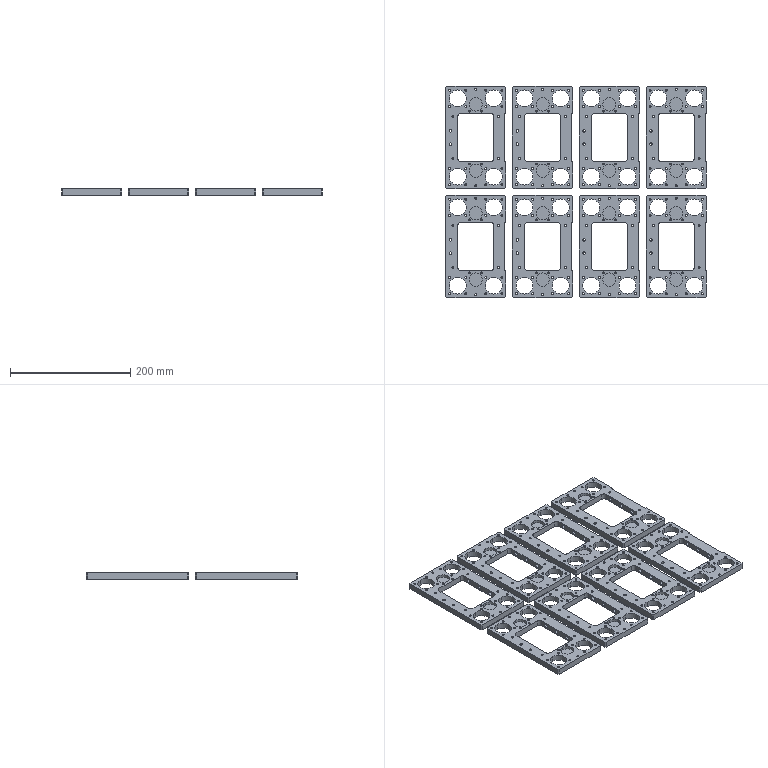NC program | NX | posted with a generic post | part box 433 x 351 x 10 mm
Lines 10233 to 11306 of 15742:
(PLANAR_MILL_COPY_COPY_COPY , TOOL : D6A45)
N20428 T01 M6
N20430 G54
N20432 G17 G0 G90 X26.9 Y-89.634 B0. C0. S9500 M3
N20434 G43 Z30. H1
N20436 Z0.5
N20438 G94 G1 Z-1. F1250.
N20440 G3 X26.4 Y-90.5 R1.
N20442 G1 Y-125.5
N20444 G3 X30.5 Y-129.6 R4.1
N20446 G1 X80.5
N20448 G3 X84.6 Y-125.5 R4.1
N20450 G1 Y-55.5
N20452 G3 X80.5 Y-51.4 R4.1
N20454 G1 X30.5
N20456 G3 X26.4 Y-55.5 R4.1
N20458 G1 Y-90.5
N20460 G3 X26.9 Y-91.366 R1.
N20462 G1 Z0.5
N20464 G0 Z30.
N20466 X4.1
N20468 Z0.5
N20470 G1 Z-1.
N20472 G3 X4.6 Y-90.5 R1.
N20474 G1 Y-7.5
N20476 G2 X4.864 Y-6.864 R0.9
N20478 G1 X6.864 Y-4.864
N20480 G2 X7.5 Y-4.6 R0.9
N20482 G1 X103.5
N20484 G2 X104.136 Y-4.864 R0.9
N20486 G1 X106.136 Y-6.864
N20488 G2 X106.4 Y-7.5 R0.9
N20490 G1 Y-50.5
N20492 G2 X105.5 Y-51.4 R0.9
N20494 G1 X104.4
N20496 Y-129.6
N20498 X105.5
N20500 G2 X106.4 Y-130.5 R0.9
N20502 G1 Y-173.5
N20504 G2 X106.136 Y-174.136 R0.9
N20506 G1 X104.136 Y-176.136
N20508 G2 X103.5 Y-176.4 R0.9
N20510 G1 X7.5
N20512 G2 X6.864 Y-176.136 R0.9
N20514 G1 X4.864 Y-174.136
N20516 G2 X4.6 Y-173.5 R0.9
N20518 G1 Y-90.5
N20520 G3 X4.1 Y-89.634 R1.
N20522 G1 Z0.5
N20524 G0 Z30.
N20526 X12.634 Y-102.2
N20528 Z0.5
N20530 G1 Z-1.
N20532 G3 X13.5 Y-102.7 R1.
N20534 X14.7 Y-101.5 R1.2
N20536 X13.5 Y-102.7 R-1.2
N20538 X14.366 Y-102.2 R1.
N20540 G1 Z0.5
N20542 G0 Z30.
N20544 X12.634 Y-80.2
N20546 Z0.5
N20548 G1 Z-1.
N20550 G3 X13.5 Y-80.7 R1.
N20552 X14.7 Y-79.5 R1.2
N20554 X13.5 Y-80.7 R-1.2
N20556 X14.366 Y-80.2 R1.
N20558 G1 Z0.5
N20560 G0 Z30.
N20562 X17.067 Y-56.
N20564 Z0.5
N20566 G1 Z-1.
N20568 G3 X17.5 Y-56.25 R0.5
N20570 X18.25 Y-55.5 R0.75
N20572 X17.5 Y-56.25 R-0.75
N20574 X17.933 Y-56. R0.5
N20576 G1 Z0.5
N20578 G0 Z30.
N20580 X11.632 Y-39.435
N20582 Z0.5
N20584 G1 Z-1.
N20586 G3 X12.065 Y-39.685 R0.5
N20588 X12.815 Y-38.935 R0.75
N20590 X12.065 Y-39.685 R-0.75
N20592 X12.498 Y-39.435 R0.5
N20594 G1 Z0.5
N20596 G0 Z30.
N20598 X-12.498
N20600 Z0.5
N20602 G1 Z-1.
N20604 G3 X-12.065 Y-39.685 R0.5
N20606 X-11.315 Y-38.935 R0.75
N20608 X-12.065 Y-39.685 R-0.75
N20610 X-11.632 Y-39.435 R0.5
N20612 G1 Z0.5
N20614 G0 Z30.
N20616 X-17.933 Y-56.
N20618 Z0.5
N20620 G1 Z-1.
N20622 G3 X-17.5 Y-56.25 R0.5
N20624 X-16.75 Y-55.5 R0.75
N20626 X-17.5 Y-56.25 R-0.75
N20628 X-17.067 Y-56. R0.5
N20630 G1 Z0.5
N20632 G0 Z30.
N20634 X-39.368 Y-39.435
N20636 Z0.5
N20638 G1 Z-1.
N20640 G3 X-38.935 Y-39.685 R0.5
N20642 X-38.185 Y-38.935 R0.75
N20644 X-38.935 Y-39.685 R-0.75
N20646 X-38.502 Y-39.435 R0.5
N20648 G1 Z0.5
N20650 G0 Z30.
N20652 X-45.933 Y-47.
N20654 Z0.5
N20656 G1 Z-1.
N20658 G3 X-45.5 Y-47.25 R0.5
N20660 X-44.75 Y-46.5 R0.75
N20662 X-45.5 Y-47.25 R-0.75
N20664 X-45.067 Y-47. R0.5
N20666 G1 Z0.5
N20668 G0 Z30.
N20670 X-56.366 Y-45.1
N20672 Z0.5
N20674 G1 Z-1.
N20676 G3 X-55.5 Y-45.6 R1.
N20678 X-45.4 Y-35.5 R10.1
N20680 X-55.5 Y-45.6 R-10.1
N20682 X-54.634 Y-45.1 R1.
N20684 G1 Z0.5
N20686 G0 Z30.
N20688 X-72.498 Y-39.435
N20690 Z0.5
N20692 G1 Z-1.
N20694 G3 X-72.065 Y-39.685 R0.5
N20696 X-71.315 Y-38.935 R0.75
N20698 X-72.065 Y-39.685 R-0.75
N20700 X-71.632 Y-39.435 R0.5
N20702 G1 Z0.5
N20704 G0 Z30.
N20706 X-65.933 Y-47.
N20708 Z0.5
N20710 G1 Z-1.
N20712 G3 X-65.5 Y-47.25 R0.5
N20714 X-64.75 Y-46.5 R0.75
N20716 X-65.5 Y-47.25 R-0.75
N20718 X-65.067 Y-47. R0.5
N20720 G1 Z0.5
N20722 G0 Z30.
N20724 X-84.1 Y-89.634
N20726 Z0.5
N20728 G1 Z-1.
N20730 G3 X-84.6 Y-90.5 R1.
N20732 G1 Y-125.5
N20734 G3 X-80.5 Y-129.6 R4.1
N20736 G1 X-30.5
N20738 G3 X-26.4 Y-125.5 R4.1
N20740 G1 Y-55.5
N20742 G3 X-30.5 Y-51.4 R4.1
N20744 G1 X-80.5
N20746 G3 X-84.6 Y-55.5 R4.1
N20748 G1 Y-90.5
N20750 G3 X-84.1 Y-91.366 R1.
N20752 G1 Z0.5
N20754 G0 Z30.
N20756 X-106.9
N20758 Z0.5
N20760 G1 Z-1.
N20762 G3 X-106.4 Y-90.5 R1.
N20764 G1 Y-7.5
N20766 G2 X-106.136 Y-6.864 R0.9
N20768 G1 X-104.136 Y-4.864
N20770 G2 X-103.5 Y-4.6 R0.9
N20772 G1 X-7.5
N20774 G2 X-6.864 Y-4.864 R0.9
N20776 G1 X-4.864 Y-6.864
N20778 G2 X-4.6 Y-7.5 R0.9
N20780 G1 Y-50.5
N20782 G2 X-5.5 Y-51.4 R0.9
N20784 G1 X-6.6
N20786 Y-129.6
N20788 X-5.5
N20790 G2 X-4.6 Y-130.5 R0.9
N20792 G1 Y-173.5
N20794 G2 X-4.864 Y-174.136 R0.9
N20796 G1 X-6.864 Y-176.136
N20798 G2 X-7.5 Y-176.4 R0.9
N20800 G1 X-103.5
N20802 G2 X-104.136 Y-176.136 R0.9
N20804 G1 X-106.136 Y-174.136
N20806 G2 X-106.4 Y-173.5 R0.9
N20808 G1 Y-90.5
N20810 G3 X-106.9 Y-89.634 R1.
N20812 G1 Z0.5
N20814 G0 Z30.
N20816 X-98.366 Y-80.2
N20818 Z0.5
N20820 G1 Z-1.
N20822 G3 X-97.5 Y-80.7 R1.
N20824 X-96.3 Y-79.5 R1.2
N20826 X-97.5 Y-80.7 R-1.2
N20828 X-96.634 Y-80.2 R1.
N20830 G1 Z0.5
N20832 G0 Z30.
N20834 X-98.366 Y-102.2
N20836 Z0.5
N20838 G1 Z-1.
N20840 G3 X-97.5 Y-102.7 R1.
N20842 X-96.3 Y-101.5 R1.2
N20844 X-97.5 Y-102.7 R-1.2
N20846 X-96.634 Y-102.2 R1.
N20848 G1 Z0.5
N20850 G0 Z30.
N20852 X-93.933 Y-126.
N20854 Z0.5
N20856 G1 Z-1.
N20858 G3 X-93.5 Y-126.25 R0.5
N20860 X-92.75 Y-125.5 R0.75
N20862 X-93.5 Y-126.25 R-0.75
N20864 X-93.067 Y-126. R0.5
N20866 G1 Z0.5
N20868 G0 Z30.
N20870 X-99.368 Y-142.565
N20872 Z0.5
N20874 G1 Z-1.
N20876 G3 X-98.935 Y-142.815 R0.5
N20878 X-98.185 Y-142.065 R0.75
N20880 X-98.935 Y-142.815 R-0.75
N20882 X-98.502 Y-142.565 R0.5
N20884 G1 Z0.5
N20886 G0 Z30.
N20888 X-86.366 Y-168.15
N20890 Z0.5
N20892 G1 Z-1.
N20894 G3 X-85.5 Y-168.65 R1.
N20896 X-72.35 Y-155.5 R13.15
N20898 X-85.5 Y-168.65 R-13.15
N20900 X-84.634 Y-168.15 R1.
N20902 G1 Z0.5
N20904 G0 Z30.
N20906 X-72.498 Y-142.565
N20908 Z0.5
N20910 G1 Z-1.
N20912 G3 X-72.065 Y-142.815 R0.5
N20914 X-71.315 Y-142.065 R0.75
N20916 X-72.065 Y-142.815 R-0.75
N20918 X-71.632 Y-142.565 R0.5
N20920 G1 Z0.5
N20922 G0 Z30.
N20924 X-65.933 Y-135.
N20926 Z0.5
N20928 G1 Z-1.
N20930 G3 X-65.5 Y-135.25 R0.5
N20932 X-64.75 Y-134.5 R0.75
N20934 X-65.5 Y-135.25 R-0.75
N20936 X-65.067 Y-135. R0.5
N20938 G1 Z0.5
N20940 G0 Z30.
N20942 X-56.366 Y-155.1
N20944 Z0.5
N20946 G1 Z-1.
N20948 G3 X-55.5 Y-155.6 R1.
N20950 X-45.4 Y-145.5 R10.1
N20952 X-55.5 Y-155.6 R-10.1
N20954 X-54.634 Y-155.1 R1.
N20956 G1 Z0.5
N20958 G0 Z30.
N20960 X-45.933 Y-135.
N20962 Z0.5
N20964 G1 Z-1.
N20966 G3 X-45.5 Y-135.25 R0.5
N20968 X-44.75 Y-134.5 R0.75
N20970 X-45.5 Y-135.25 R-0.75
N20972 X-45.067 Y-135. R0.5
N20974 G1 Z0.5
N20976 G0 Z30.
N20978 X-39.368 Y-142.565
N20980 Z0.5
N20982 G1 Z-1.
N20984 G3 X-38.935 Y-142.815 R0.5
N20986 X-38.185 Y-142.065 R0.75
N20988 X-38.935 Y-142.815 R-0.75
N20990 X-38.502 Y-142.565 R0.5
N20992 G1 Z0.5
N20994 G0 Z30.
N20996 X-17.933 Y-126.
N20998 Z0.5
N21000 G1 Z-1.
N21002 G3 X-17.5 Y-126.25 R0.5
N21004 X-16.75 Y-125.5 R0.75
N21006 X-17.5 Y-126.25 R-0.75
N21008 X-17.067 Y-126. R0.5
N21010 G1 Z0.5
N21012 G0 Z30.
N21014 X-12.498 Y-142.565
N21016 Z0.5
N21018 G1 Z-1.
N21020 G3 X-12.065 Y-142.815 R0.5
N21022 X-11.315 Y-142.065 R0.75
N21024 X-12.065 Y-142.815 R-0.75
N21026 X-11.632 Y-142.565 R0.5
N21028 G1 Z0.5
N21030 G0 Z30.
N21032 X17.067 Y-126.
N21034 Z0.5
N21036 G1 Z-1.
N21038 G3 X17.5 Y-126.25 R0.5
N21040 X18.25 Y-125.5 R0.75
N21042 X17.5 Y-126.25 R-0.75
N21044 X17.933 Y-126. R0.5
N21046 G1 Z0.5
N21048 G0 Z30.
N21050 X11.632 Y-142.565
N21052 Z0.5
N21054 G1 Z-1.
N21056 G3 X12.065 Y-142.815 R0.5
N21058 X12.815 Y-142.065 R0.75
N21060 X12.065 Y-142.815 R-0.75
N21062 X12.498 Y-142.565 R0.5
N21064 G1 Z0.5
N21066 G0 Z30.
N21068 X24.634 Y-168.15
N21070 Z0.5
N21072 G1 Z-1.
N21074 G3 X25.5 Y-168.65 R1.
N21076 X38.65 Y-155.5 R13.15
N21078 X25.5 Y-168.65 R-13.15
N21080 X26.366 Y-168.15 R1.
N21082 G1 Z0.5
N21084 G0 Z30.
N21086 X38.502 Y-142.565
N21088 Z0.5
N21090 G1 Z-1.
N21092 G3 X38.935 Y-142.815 R0.5
N21094 X39.685 Y-142.065 R0.75
N21096 X38.935 Y-142.815 R-0.75
N21098 X39.368 Y-142.565 R0.5
N21100 G1 Z0.5
N21102 G0 Z30.
N21104 X45.067 Y-135.
N21106 Z0.5
N21108 G1 Z-1.
N21110 G3 X45.5 Y-135.25 R0.5
N21112 X46.25 Y-134.5 R0.75
N21114 X45.5 Y-135.25 R-0.75
N21116 X45.933 Y-135. R0.5
N21118 G1 Z0.5
N21120 G0 Z30.
N21122 X54.634 Y-155.1
N21124 Z0.5
N21126 G1 Z-1.
N21128 G3 X55.5 Y-155.6 R1.
N21130 X65.6 Y-145.5 R10.1
N21132 X55.5 Y-155.6 R-10.1
N21134 X56.366 Y-155.1 R1.
N21136 G1 Z0.5
N21138 G0 Z30.
N21140 X65.067 Y-135.
N21142 Z0.5
N21144 G1 Z-1.
N21146 G3 X65.5 Y-135.25 R0.5
N21148 X66.25 Y-134.5 R0.75
N21150 X65.5 Y-135.25 R-0.75
N21152 X65.933 Y-135. R0.5
N21154 G1 Z0.5
N21156 G0 Z30.
N21158 X71.632 Y-142.565
N21160 Z0.5
N21162 G1 Z-1.
N21164 G3 X72.065 Y-142.815 R0.5
N21166 X72.815 Y-142.065 R0.75
N21168 X72.065 Y-142.815 R-0.75
N21170 X72.498 Y-142.565 R0.5
N21172 G1 Z0.5
N21174 G0 Z30.
N21176 X98.502
N21178 Z0.5
N21180 G1 Z-1.
N21182 G3 X98.935 Y-142.815 R0.5
N21184 X99.685 Y-142.065 R0.75
N21186 X98.935 Y-142.815 R-0.75
N21188 X99.368 Y-142.565 R0.5
N21190 G1 Z0.5
N21192 G0 Z30.
N21194 X93.067 Y-126.
N21196 Z0.5
N21198 G1 Z-1.
N21200 G3 X93.5 Y-126.25 R0.5
N21202 X94.25 Y-125.5 R0.75
N21204 X93.5 Y-126.25 R-0.75
N21206 X93.933 Y-126. R0.5
N21208 G1 Z0.5
N21210 G0 Z30.
N21212 X122.632 Y-142.565
N21214 Z0.5
N21216 G1 Z-1.
N21218 G3 X123.065 Y-142.815 R0.5
N21220 X123.815 Y-142.065 R0.75
N21222 X123.065 Y-142.815 R-0.75
N21224 X123.498 Y-142.565 R0.5
N21226 G1 Z0.5
N21228 G0 Z30.
N21230 X128.067 Y-126.
N21232 Z0.5
N21234 G1 Z-1.
N21236 G3 X128.5 Y-126.25 R0.5
N21238 X129.25 Y-125.5 R0.75
N21240 X128.5 Y-126.25 R-0.75
N21242 X128.933 Y-126. R0.5
N21244 G1 Z0.5
N21246 G0 Z30.
N21248 X123.634 Y-102.2
N21250 Z0.5
N21252 G1 Z-1.
N21254 G3 X124.5 Y-102.7 R1.
N21256 X125.7 Y-101.5 R1.2
N21258 X124.5 Y-102.7 R-1.2
N21260 X125.366 Y-102.2 R1.
N21262 G1 Z0.5
N21264 G0 Z30.
N21266 X125.2 Y-80.366
N21268 Z0.5
N21270 G1 Z-1.
N21272 G3 X125.7 Y-79.5 R1.
N21274 X124.5 Y-78.3 R1.2
N21276 X125.7 Y-79.5 R-1.2
N21278 X125.2 Y-78.634 R1.
N21280 G1 Z0.5
N21282 G0 Z30.
N21284 X129. Y-55.933
N21286 Z0.5
N21288 G1 Z-1.
N21290 G3 X129.25 Y-55.5 R0.5
N21292 X128.5 Y-54.75 R0.75
N21294 X129.25 Y-55.5 R-0.75
N21296 X129. Y-55.067 R0.5
N21298 G1 Z0.5
N21300 G0 Z30.
N21302 X123.565 Y-39.368
N21304 Z0.5
N21306 G1 Z-1.
N21308 G3 X123.815 Y-38.935 R0.5
N21310 X123.065 Y-38.185 R0.75
N21312 X123.815 Y-38.935 R-0.75
N21314 X123.565 Y-38.502 R0.5
N21316 G1 Z0.5
N21318 G0 Z30.
N21320 X149.15 Y-26.366
N21322 Z0.5
N21324 G1 Z-1.
N21326 G3 X149.65 Y-25.5 R1.
N21328 X136.5 Y-12.35 R13.15
N21330 X149.65 Y-25.5 R-13.15
N21332 X149.15 Y-24.634 R1.
N21334 G1 Z0.5
N21336 G0 Z30.
N21338 X123.565 Y-12.498
N21340 Z0.5
N21342 G1 Z-1.
N21344 G3 X123.815 Y-12.065 R0.5
N21346 X123.065 Y-11.315 R0.75
N21348 X123.815 Y-12.065 R-0.75
N21350 X123.565 Y-11.632 R0.5
N21352 G1 Z0.5
N21354 G0 Z30.
N21356 Y11.632
N21358 Z0.5
N21360 G1 Z-1.
N21362 G3 X123.815 Y12.065 R0.5
N21364 X123.065 Y12.815 R0.75
N21366 X123.815 Y12.065 R-0.75
N21368 X123.565 Y12.498 R0.5
N21370 G1 Z0.5
N21372 G0 Z30.
N21374 X99.435 Y11.632
N21376 Z0.5
N21378 G1 Z-1.
N21380 G3 X99.685 Y12.065 R0.5
N21382 X98.935 Y12.815 R0.75
N21384 X99.685 Y12.065 R-0.75
N21386 X99.435 Y12.498 R0.5
N21388 G1 Z0.5
N21390 G0 Z30.
N21392 Y-12.498
N21394 Z0.5
N21396 G1 Z-1.
N21398 G3 X99.685 Y-12.065 R0.5
N21400 X98.935 Y-11.315 R0.75
N21402 X99.685 Y-12.065 R-0.75
N21404 X99.435 Y-11.632 R0.5
N21406 G1 Z0.5
N21408 G0 Z30.
N21410 X98.15 Y-26.366
N21412 Z0.5
N21414 G1 Z-1.
N21416 G3 X98.65 Y-25.5 R1.
N21418 X85.5 Y-12.35 R13.15
N21420 X98.65 Y-25.5 R-13.15
N21422 X98.15 Y-24.634 R1.
N21424 G1 Z0.5
N21426 G0 Z30.
N21428 X99.435 Y-39.368
N21430 Z0.5
N21432 G1 Z-1.
N21434 G3 X99.685 Y-38.935 R0.5
N21436 X98.935 Y-38.185 R0.75
N21438 X99.685 Y-38.935 R-0.75
N21440 X99.435 Y-38.502 R0.5
N21442 G1 Z0.5
N21444 G0 Z30.
N21446 X93.067 Y-56.
N21448 Z0.5
N21450 G1 Z-1.
N21452 G3 X93.5 Y-56.25 R0.5
N21454 X94.25 Y-55.5 R0.75
N21456 X93.5 Y-56.25 R-0.75
N21458 X93.933 Y-56. R0.5
N21460 G1 Z0.5
N21462 G0 Z30.
N21464 X71.632 Y-39.435
N21466 Z0.5
N21468 G1 Z-1.
N21470 G3 X72.065 Y-39.685 R0.5
N21472 X72.815 Y-38.935 R0.75
N21474 X72.065 Y-39.685 R-0.75
N21476 X72.498 Y-39.435 R0.5
N21478 G1 Z0.5
N21480 G0 Z30.
N21482 X65.067 Y-47.
N21484 Z0.5
N21486 G1 Z-1.
N21488 G3 X65.5 Y-47.25 R0.5
N21490 X66.25 Y-46.5 R0.75
N21492 X65.5 Y-47.25 R-0.75
N21494 X65.933 Y-47. R0.5
N21496 G1 Z0.5
N21498 G0 Z30.
N21500 X45.067
N21502 Z0.5
N21504 G1 Z-1.
N21506 G3 X45.5 Y-47.25 R0.5
N21508 X46.25 Y-46.5 R0.75
N21510 X45.5 Y-47.25 R-0.75
N21512 X45.933 Y-47. R0.5
N21514 G1 Z0.5
N21516 G0 Z30.
N21518 X38.502 Y-39.435
N21520 Z0.5
N21522 G1 Z-1.
N21524 G3 X38.935 Y-39.685 R0.5
N21526 X39.685 Y-38.935 R0.75
N21528 X38.935 Y-39.685 R-0.75
N21530 X39.368 Y-39.435 R0.5
N21532 G1 Z0.5
N21534 G0 Z30.
N21536 X54.634 Y-45.1
N21538 Z0.5
N21540 G1 Z-1.
N21542 G3 X55.5 Y-45.6 R1.
N21544 X65.6 Y-35.5 R10.1
N21546 X55.5 Y-45.6 R-10.1
N21548 X56.366 Y-45.1 R1.
N21550 G1 Z0.5
N21552 G0 Z30.
N21554 X72.565 Y-12.498
N21556 Z0.5
N21558 G1 Z-1.
N21560 G3 X72.815 Y-12.065 R0.5
N21562 X72.065 Y-11.315 R0.75
N21564 X72.815 Y-12.065 R-0.75
N21566 X72.565 Y-11.632 R0.5
N21568 G1 Z0.5
N21570 G0 Z30.
N21572 X56. Y-10.933
N21574 Z0.5
N21576 G1 Z-1.
N21578 G3 X56.25 Y-10.5 R0.5
N21580 X55.5 Y-9.75 R0.75
N21582 X56.25 Y-10.5 R-0.75
N21584 X56. Y-10.067 R0.5
N21586 G1 Z0.5
N21588 G0 Z30.
N21590 X38.502 Y-12.565
N21592 Z0.5
N21594 G1 Z-1.
N21596 G3 X38.935 Y-12.815 R0.5
N21598 X39.685 Y-12.065 R0.75
N21600 X38.935 Y-12.815 R-0.75
N21602 X39.368 Y-12.565 R0.5
N21604 G1 Z0.5
N21606 G0 Z30.
N21608 X24.634 Y-38.15
N21610 Z0.5
N21612 G1 Z-1.
N21614 G3 X25.5 Y-38.65 R1.
N21616 X38.65 Y-25.5 R13.15
N21618 X25.5 Y-38.65 R-13.15
N21620 X26.366 Y-38.15 R1.
N21622 G1 Z0.5
N21624 G0 Z30.
N21626 X11.632 Y-12.565
N21628 Z0.5
N21630 G1 Z-1.
N21632 G3 X12.065 Y-12.815 R0.5
N21634 X12.815 Y-12.065 R0.75
N21636 X12.065 Y-12.815 R-0.75
N21638 X12.498 Y-12.565 R0.5
N21640 G1 Z0.5
N21642 G0 Z30.
N21644 X-12.498
N21646 Z0.5
N21648 G1 Z-1.
N21650 G3 X-12.065 Y-12.815 R0.5
N21652 X-11.315 Y-12.065 R0.75
N21654 X-12.065 Y-12.815 R-0.75
N21656 X-11.632 Y-12.565 R0.5
N21658 G1 Z0.5
N21660 G0 Z30.
N21662 X-26.366 Y-38.15
N21664 Z0.5
N21666 G1 Z-1.
N21668 G3 X-25.5 Y-38.65 R1.
N21670 X-12.35 Y-25.5 R13.15
N21672 X-25.5 Y-38.65 R-13.15
N21674 X-24.634 Y-38.15 R1.
N21676 G1 Z0.5
N21678 G0 Z30.
N21680 X-39.368 Y-12.565
N21682 Z0.5
N21684 G1 Z-1.
N21686 G3 X-38.935 Y-12.815 R0.5
N21688 X-38.185 Y-12.065 R0.75
N21690 X-38.935 Y-12.815 R-0.75
N21692 X-38.502 Y-12.565 R0.5
N21694 G1 Z0.5
N21696 G0 Z30.
N21698 X-56. Y-10.067
N21700 Z0.5
N21702 G1 Z-1.
N21704 G3 X-56.25 Y-10.5 R0.5
N21706 X-55.5 Y-11.25 R0.75
N21708 X-56.25 Y-10.5 R-0.75
N21710 X-56. Y-10.933 R0.5
N21712 G1 Z0.5
N21714 G0 Z30.
N21716 X-72.565 Y-11.632
N21718 Z0.5
N21720 G1 Z-1.
N21722 G3 X-72.815 Y-12.065 R0.5
N21724 X-72.065 Y-12.815 R0.75
N21726 X-72.815 Y-12.065 R-0.75
N21728 X-72.565 Y-12.498 R0.5
N21730 G1 Z0.5
N21732 G0 Z30.
N21734 X-98.15 Y-24.634
N21736 Z0.5
N21738 G1 Z-1.
N21740 G3 X-98.65 Y-25.5 R1.
N21742 X-85.5 Y-38.65 R13.15
N21744 X-98.65 Y-25.5 R-13.15
N21746 X-98.15 Y-26.366 R1.
N21748 G1 Z0.5
N21750 G0 Z30.
N21752 X-99.435 Y-11.632
N21754 Z0.5
N21756 G1 Z-1.
N21758 G3 X-99.685 Y-12.065 R0.5
N21760 X-98.935 Y-12.815 R0.75
N21762 X-99.685 Y-12.065 R-0.75
N21764 X-99.435 Y-12.498 R0.5
N21766 G1 Z0.5
N21768 G0 Z30.
N21770 Y-38.502
N21772 Z0.5
N21774 G1 Z-1.
N21776 G3 X-99.685 Y-38.935 R0.5
N21778 X-98.935 Y-39.685 R0.75
N21780 X-99.685 Y-38.935 R-0.75
N21782 X-99.435 Y-39.368 R0.5
N21784 G1 Z0.5
N21786 G0 Z30.
N21788 X-93.933 Y-56.
N21790 Z0.5
N21792 G1 Z-1.
N21794 G3 X-93.5 Y-56.25 R0.5
N21796 X-92.75 Y-55.5 R0.75
N21798 X-93.5 Y-56.25 R-0.75
N21800 X-93.067 Y-56. R0.5
N21802 G1 Z0.5
N21804 G0 Z30.
N21806 X-123.565 Y-38.502
N21808 Z0.5
N21810 G1 Z-1.
N21812 G3 X-123.815 Y-38.935 R0.5
N21814 X-123.065 Y-39.685 R0.75
N21816 X-123.815 Y-38.935 R-0.75
N21818 X-123.565 Y-39.368 R0.5
N21820 G1 Z0.5
N21822 G0 Z30.
N21824 X-129. Y-55.067
N21826 Z0.5
N21828 G1 Z-1.
N21830 G3 X-129.25 Y-55.5 R0.5
N21832 X-128.5 Y-56.25 R0.75
N21834 X-129.25 Y-55.5 R-0.75
N21836 X-129. Y-55.933 R0.5
N21838 G1 Z0.5
N21840 G0 Z30.
N21842 X-195.1 Y-89.634
N21844 Z0.5
N21846 G1 Z-1.
N21848 G3 X-195.6 Y-90.5 R1.
N21850 G1 Y-125.5
N21852 G3 X-191.5 Y-129.6 R4.1
N21854 G1 X-141.5
N21856 G3 X-137.4 Y-125.5 R4.1
N21858 G1 Y-55.5
N21860 G3 X-141.5 Y-51.4 R4.1
N21862 G1 X-191.5
N21864 G3 X-195.6 Y-55.5 R4.1
N21866 G1 Y-90.5
N21868 G3 X-195.1 Y-91.366 R1.
N21870 G1 Z0.5
N21872 G0 Z30.
N21874 X-217.9
N21876 Z0.5
N21878 G1 Z-1.
N21880 G3 X-217.4 Y-90.5 R1.
N21882 G1 Y-7.5
N21884 G2 X-217.136 Y-6.864 R0.9
N21886 G1 X-215.136 Y-4.864
N21888 G2 X-214.5 Y-4.6 R0.9
N21890 G1 X-118.5
N21892 G2 X-117.864 Y-4.864 R0.9
N21894 G1 X-115.864 Y-6.864
N21896 G2 X-115.6 Y-7.5 R0.9
N21898 G1 Y-50.5
N21900 G2 X-116.5 Y-51.4 R0.9
N21902 G1 X-117.6
N21904 Y-129.6
N21906 X-116.5
N21908 G2 X-115.6 Y-130.5 R0.9
N21910 G1 Y-173.5
N21912 G2 X-115.864 Y-174.136 R0.9
N21914 G1 X-117.864 Y-176.136
N21916 G2 X-118.5 Y-176.4 R0.9
N21918 G1 X-214.5
N21920 G2 X-215.136 Y-176.136 R0.9
N21922 G1 X-217.136 Y-174.136
N21924 G2 X-217.4 Y-173.5 R0.9
N21926 G1 Y-90.5
N21928 G3 X-217.9 Y-89.634 R1.
N21930 G1 Z0.5
N21932 G0 Z30.
N21934 X-209.2 Y-78.634
N21936 Z0.5
N21938 G1 Z-1.
N21940 G3 X-209.7 Y-79.5 R1.
N21942 X-208.5 Y-80.7 R1.2
N21944 X-209.7 Y-79.5 R-1.2
N21946 X-209.2 Y-80.366 R1.
N21948 G1 Z0.5
N21950 G0 Z30.
N21952 Y-100.634
N21954 Z0.5
N21956 G1 Z-1.
N21958 G3 X-209.7 Y-101.5 R1.
N21960 X-208.5 Y-102.7 R1.2
N21962 X-209.7 Y-101.5 R-1.2
N21964 X-209.2 Y-102.366 R1.
N21966 G1 Z0.5
N21968 G0 Z30.
N21970 X-205. Y-125.067
N21972 Z0.5
N21974 G1 Z-1.
N21976 G3 X-205.25 Y-125.5 R0.5
N21978 X-204.5 Y-126.25 R0.75
N21980 X-205.25 Y-125.5 R-0.75
N21982 X-205. Y-125.933 R0.5
N21984 G1 Z0.5
N21986 G0 Z30.
N21988 X-210.435 Y-141.632
N21990 Z0.5
N21992 G1 Z-1.
N21994 G3 X-210.685 Y-142.065 R0.5
N21996 X-209.935 Y-142.815 R0.75
N21998 X-210.685 Y-142.065 R-0.75
N22000 X-210.435 Y-142.498 R0.5
N22002 G1 Z0.5
N22004 G0 Z30.
N22006 Y-168.502
N22008 Z0.5
N22010 G1 Z-1.
N22012 G3 X-210.685 Y-168.935 R0.5
N22014 X-209.935 Y-169.685 R0.75
N22016 X-210.685 Y-168.935 R-0.75
N22018 X-210.435 Y-169.368 R0.5
N22020 G1 Z0.5
N22022 G0 Z30.
N22024 X-197.366 Y-168.15
N22026 Z0.5
N22028 G1 Z-1.
N22030 G3 X-196.5 Y-168.65 R1.
N22032 X-183.35 Y-155.5 R13.15
N22034 X-196.5 Y-168.65 R-13.15
N22036 X-195.634 Y-168.15 R1.
N22038 G1 Z0.5
N22040 G0 Z30.
N22042 X-183.498 Y-142.565
N22044 Z0.5
N22046 G1 Z-1.
N22048 G3 X-183.065 Y-142.815 R0.5
N22050 X-182.315 Y-142.065 R0.75
N22052 X-183.065 Y-142.815 R-0.75
N22054 X-182.632 Y-142.565 R0.5
N22056 G1 Z0.5
N22058 G0 Z30.
N22060 X-177. Y-134.067
N22062 Z0.5
N22064 G1 Z-1.
N22066 G3 X-177.25 Y-134.5 R0.5
N22068 X-176.5 Y-135.25 R0.75
N22070 X-177.25 Y-134.5 R-0.75
N22072 X-177. Y-134.933 R0.5
N22074 G1 Z0.5
N22076 G0 Z30.
N22078 X-156.933 Y-135.
N22080 Z0.5
N22082 G1 Z-1.
N22084 G3 X-156.5 Y-135.25 R0.5
N22086 X-155.75 Y-134.5 R0.75
N22088 X-156.5 Y-135.25 R-0.75
N22090 X-156.067 Y-135. R0.5
N22092 G1 Z0.5
N22094 G0 Z30.
N22096 X-167.366 Y-155.1
N22098 Z0.5
N22100 G1 Z-1.
N22102 G3 X-166.5 Y-155.6 R1.
N22104 X-156.4 Y-145.5 R10.1
N22106 X-166.5 Y-155.6 R-10.1
N22108 X-165.634 Y-155.1 R1.
N22110 G1 Z0.5
N22112 G0 Z30.
N22114 X-183.498 Y-169.435
N22116 Z0.5
N22118 G1 Z-1.
N22120 G3 X-183.065 Y-169.685 R0.5
N22122 X-182.315 Y-168.935 R0.75
N22124 X-183.065 Y-169.685 R-0.75
N22126 X-182.632 Y-169.435 R0.5
N22128 G1 Z0.5
N22130 G0 Z30.
N22132 X-166.933 Y-171.
N22134 Z0.5
N22136 G1 Z-1.
N22138 G3 X-166.5 Y-171.25 R0.5
N22140 X-165.75 Y-170.5 R0.75
N22142 X-166.5 Y-171.25 R-0.75
N22144 X-166.067 Y-171. R0.5
N22146 G1 Z0.5
N22148 G0 Z30.
N22150 X-150.368 Y-169.435
N22152 Z0.5
N22154 G1 Z-1.
N22156 G3 X-149.935 Y-169.685 R0.5
N22158 X-149.185 Y-168.935 R0.75
N22160 X-149.935 Y-169.685 R-0.75
N22162 X-149.502 Y-169.435 R0.5
N22164 G1 Z0.5
N22166 G0 Z30.
N22168 X-150.368 Y-142.565
N22170 Z0.5
N22172 G1 Z-1.
N22174 G3 X-149.935 Y-142.815 R0.5
N22176 X-149.185 Y-142.065 R0.75
N22178 X-149.935 Y-142.815 R-0.75
N22180 X-149.502 Y-142.565 R0.5
N22182 G1 Z0.5
N22184 G0 Z30.
N22186 X-128.933 Y-126.
N22188 Z0.5
N22190 G1 Z-1.
N22192 G3 X-128.5 Y-126.25 R0.5
N22194 X-127.75 Y-125.5 R0.75
N22196 X-128.5 Y-126.25 R-0.75
N22198 X-128.067 Y-126. R0.5
N22200 G1 Z0.5
N22202 G0 Z30.
N22204 X-123.498 Y-142.565
N22206 Z0.5
N22208 G1 Z-1.
N22210 G3 X-123.065 Y-142.815 R0.5
N22212 X-122.315 Y-142.065 R0.75
N22214 X-123.065 Y-142.815 R-0.75
N22216 X-122.632 Y-142.565 R0.5
N22218 G1 Z0.5
N22220 G0 Z30.
N22222 X-137.366 Y-168.15
N22224 Z0.5
N22226 G1 Z-1.
N22228 G3 X-136.5 Y-168.65 R1.
N22230 X-123.35 Y-155.5 R13.15
N22232 X-136.5 Y-168.65 R-13.15
N22234 X-135.634 Y-168.15 R1.
N22236 G1 Z0.5
N22238 G0 Z30.
N22240 X-123.498 Y-169.435
N22242 Z0.5
N22244 G1 Z-1.
N22246 G3 X-123.065 Y-169.685 R0.5
N22248 X-122.315 Y-168.935 R0.75
N22250 X-123.065 Y-169.685 R-0.75
N22252 X-122.632 Y-169.435 R0.5
N22254 G1 Z0.5
N22256 G0 Z30.
N22258 X-99.368
N22260 Z0.5
N22262 G1 Z-1.
N22264 G3 X-98.935 Y-169.685 R0.5
N22266 X-98.185 Y-168.935 R0.75
N22268 X-98.935 Y-169.685 R-0.75
N22270 X-98.502 Y-169.435 R0.5
N22272 G1 Z0.5
N22274 G0 Z30.
N22276 X-72.498
N22278 Z0.5
N22280 G1 Z-1.
N22282 G3 X-72.065 Y-169.685 R0.5
N22284 X-71.315 Y-168.935 R0.75
N22286 X-72.065 Y-169.685 R-0.75
N22288 X-71.632 Y-169.435 R0.5
N22290 G1 Z0.5
N22292 G0 Z30.
N22294 X-55.933 Y-171.
N22296 Z0.5
N22298 G1 Z-1.
N22300 G3 X-55.5 Y-171.25 R0.5
N22302 X-54.75 Y-170.5 R0.75
N22304 X-55.5 Y-171.25 R-0.75
N22306 X-55.067 Y-171. R0.5
N22308 G1 Z0.5
N22310 G0 Z30.
N22312 X-39.368 Y-169.435
N22314 Z0.5
N22316 G1 Z-1.
N22318 G3 X-38.935 Y-169.685 R0.5
N22320 X-38.185 Y-168.935 R0.75
N22322 X-38.935 Y-169.685 R-0.75
N22324 X-38.502 Y-169.435 R0.5
N22326 G1 Z0.5
N22328 G0 Z30.
N22330 X-26.366 Y-168.15
N22332 Z0.5
N22334 G1 Z-1.
N22336 G3 X-25.5 Y-168.65 R1.
N22338 X-12.35 Y-155.5 R13.15
N22340 X-25.5 Y-168.65 R-13.15
N22342 X-24.634 Y-168.15 R1.
N22344 G1 Z0.5
N22346 G0 Z30.
N22348 X-12.498 Y-169.435
N22350 Z0.5
N22352 G1 Z-1.
N22354 G3 X-12.065 Y-169.685 R0.5
N22356 X-11.315 Y-168.935 R0.75
N22358 X-12.065 Y-169.685 R-0.75
N22360 X-11.632 Y-169.435 R0.5
N22362 G1 Z0.5
N22364 G0 Z30.
N22366 X11.632
N22368 Z0.5
N22370 G1 Z-1.
N22372 G3 X12.065 Y-169.685 R0.5
N22374 X12.815 Y-168.935 R0.75
N22376 X12.065 Y-169.685 R-0.75
N22378 X12.498 Y-169.435 R0.5
N22380 G1 Z0.5
N22382 G0 Z30.
N22384 X38.502
N22386 Z0.5
N22388 G1 Z-1.
N22390 G3 X38.935 Y-169.685 R0.5
N22392 X39.685 Y-168.935 R0.75
N22394 X38.935 Y-169.685 R-0.75
N22396 X39.368 Y-169.435 R0.5
N22398 G1 Z0.5
N22400 G0 Z30.
N22402 X55.067 Y-171.
N22404 Z0.5
N22406 G1 Z-1.
N22408 G3 X55.5 Y-171.25 R0.5
N22410 X56.25 Y-170.5 R0.75
N22412 X55.5 Y-171.25 R-0.75
N22414 X55.933 Y-171. R0.5
N22416 G1 Z0.5
N22418 G0 Z30.
N22420 X71.632 Y-169.435
N22422 Z0.5
N22424 G1 Z-1.
N22426 G3 X72.065 Y-169.685 R0.5
N22428 X72.815 Y-168.935 R0.75
N22430 X72.065 Y-169.685 R-0.75
N22432 X72.498 Y-169.435 R0.5
N22434 G1 Z0.5
N22436 G0 Z30.
N22438 X84.634 Y-168.15
N22440 Z0.5
N22442 G1 Z-1.
N22444 G3 X85.5 Y-168.65 R1.
N22446 X98.65 Y-155.5 R13.15
N22448 X85.5 Y-168.65 R-13.15
N22450 X86.366 Y-168.15 R1.
N22452 G1 Z0.5
N22454 G0 Z30.
N22456 X98.502 Y-169.435
N22458 Z0.5
N22460 G1 Z-1.
N22462 G3 X98.935 Y-169.685 R0.5
N22464 X99.685 Y-168.935 R0.75
N22466 X98.935 Y-169.685 R-0.75
N22468 X99.368 Y-169.435 R0.5
N22470 G1 Z0.5
N22472 G0 Z30.
N22474 X122.632
N22476 Z0.5
N22478 G1 Z-1.
N22480 G3 X123.065 Y-169.685 R0.5
N22482 X123.815 Y-168.935 R0.75
N22484 X123.065 Y-169.685 R-0.75
N22486 X123.498 Y-169.435 R0.5
N22488 G1 Z0.5
N22490 G0 Z30.
N22492 X135.634 Y-168.15
N22494 Z0.5
N22496 G1 Z-1.
N22498 G3 X136.5 Y-168.65 R1.
N22500 X149.65 Y-155.5 R13.15
N22502 X136.5 Y-168.65 R-13.15
N22504 X137.366 Y-168.15 R1.
N22506 G1 Z0.5
N22508 G0 Z30.
N22510 X149.502 Y-169.435
N22512 Z0.5
N22514 G1 Z-1.
N22516 G3 X149.935 Y-169.685 R0.5
N22518 X150.685 Y-168.935 R0.75
N22520 X149.935 Y-169.685 R-0.75
N22522 X150.368 Y-169.435 R0.5
N22524 G1 Z0.5
N22526 G0 Z30.
N22528 X149.502 Y-142.565
N22530 Z0.5
N22532 G1 Z-1.
N22534 G3 X149.935 Y-142.815 R0.5
N22536 X150.685 Y-142.065 R0.75
N22538 X149.935 Y-142.815 R-0.75
N22540 X150.368 Y-142.565 R0.5
N22542 G1 Z0.5
N22544 G0 Z30.
N22546 X156.067 Y-135.
N22548 Z0.5
N22550 G1 Z-1.
N22552 G3 X156.5 Y-135.25 R0.5
N22554 X157.25 Y-134.5 R0.75
N22556 X156.5 Y-135.25 R-0.75
N22558 X156.933 Y-135. R0.5
N22560 G1 Z0.5
N22562 G0 Z30.
N22564 X165.634 Y-155.1
N22566 Z0.5
N22568 G1 Z-1.